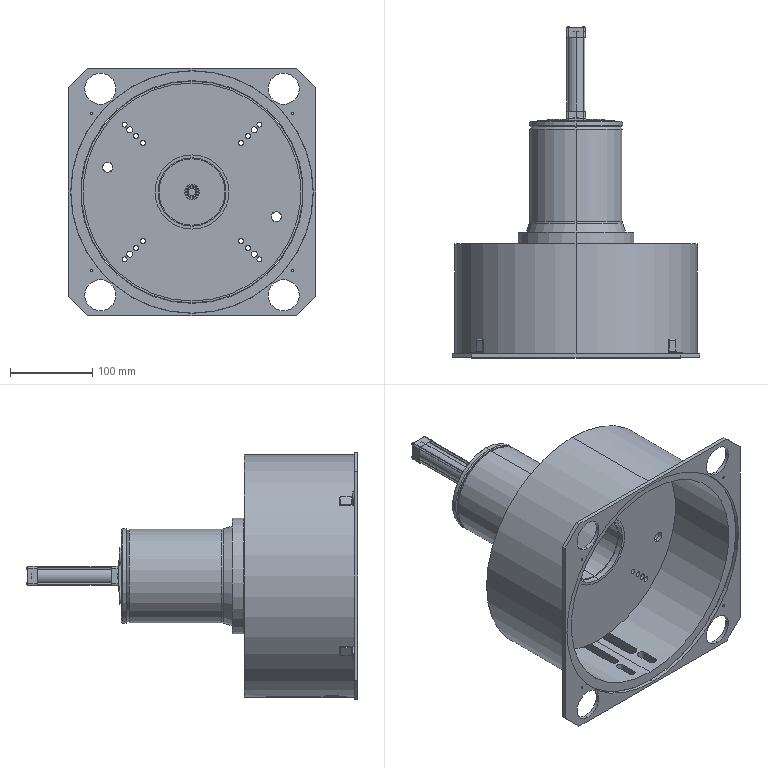Part | SolidWorks | features BaseBody 27, Scale 1 | 27 solids | 697 faces | box 300.482 x 402.788 x 300.482 mm | volume 4049858 mm3 | cylinder 456 | plane 153 | cone 68 | torus 20 | commonest cylinder face diameters 14.196 x59 2.484 x48 5.915 x40 6.01 x40 5.205 x24 2.887 x16